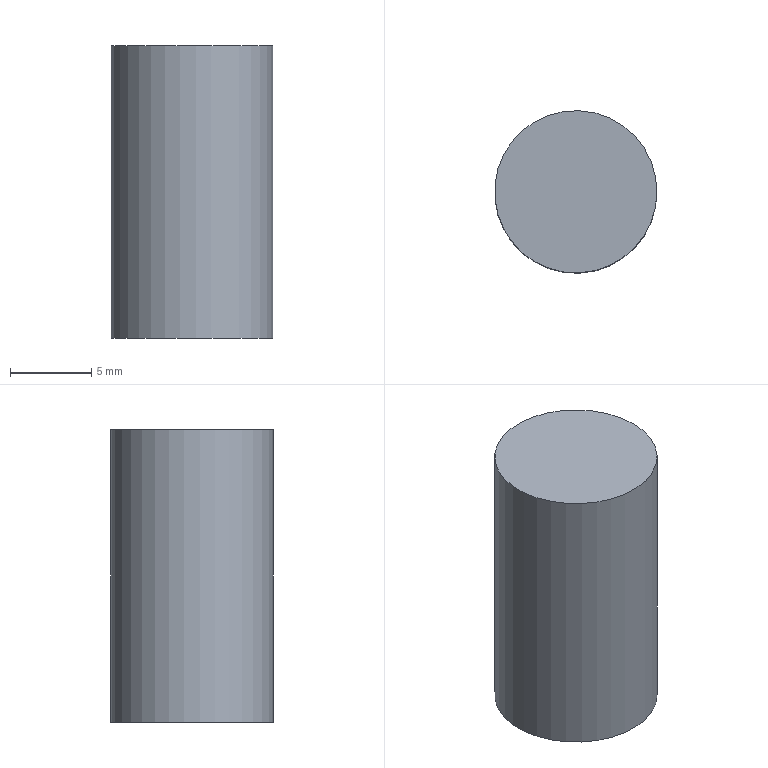Part | STEP file | xiaoding10x18 | 1 solid | 3 faces | box 10 x 10 x 18 mm | volume 1414 mm3 | plane 2 | cylinder 1 | commonest cylinder face diameters 10 x1
STEP:
#1=CARTESIAN_POINT('',(0.,0.,0.));
#2=DIRECTION('',(0.,0.,1.));
#3=DIRECTION('',(1.,0.,0.));
#4=AXIS2_PLACEMENT_3D('',#1,#2,#3);
#5=CARTESIAN_POINT('',(5.,0.,9.));
#6=VERTEX_POINT('',#5);
#7=CARTESIAN_POINT('',(0.,0.,9.));
#8=DIRECTION('',(0.,0.,1.));
#9=DIRECTION('',(1.,0.,0.));
#10=AXIS2_PLACEMENT_3D('',#7,#8,#9);
#11=CIRCLE('',#10,5.);
#12=CARTESIAN_POINT('',(0.,0.,9.));
#13=DIRECTION('',(0.,0.,-1.));
#14=DIRECTION('',(-1.,0.,0.));
#15=AXIS2_PLACEMENT_3D('',#12,#13,#14);
#16=CYLINDRICAL_SURFACE('',#15,5.);
#17=CARTESIAN_POINT('',(9.425,0.));
#18=DIRECTION('',(-1.,0.));
#19=VECTOR('',#18,1.);
#20=LINE('',#17,#19);
#21=(GEOMETRIC_REPRESENTATION_CONTEXT(2)PARAMETRIC_REPRESENTATION_CONTEXT()REPRESENTATION_CONTEXT('',''));
#22=DEFINITIONAL_REPRESENTATION('',(#20),#21);
#23=PCURVE('',#16,#22);
#24=CARTESIAN_POINT('',(0.,0.,9.));
#25=DIRECTION('',(0.,0.,1.));
#26=DIRECTION('',(1.,0.,0.));
#27=AXIS2_PLACEMENT_3D('',#24,#25,#26);
#28=PLANE('',#27);
#29=CARTESIAN_POINT('',(0.,0.));
#30=DIRECTION('',(1.,0.));
#31=AXIS2_PLACEMENT_2D('',#29,#30);
#32=CIRCLE('',#31,5.);
#33=(GEOMETRIC_REPRESENTATION_CONTEXT(2)PARAMETRIC_REPRESENTATION_CONTEXT()REPRESENTATION_CONTEXT('',''));
#34=DEFINITIONAL_REPRESENTATION('',(#32),#33);
#35=PCURVE('',#28,#34);
#36=SURFACE_CURVE('',#11,(#23,#35),.PCURVE_S1.);
#37=EDGE_CURVE('',#6,#6,#36,.T.);
#38=ORIENTED_EDGE('',*,*,#37,.F.);
#39=CARTESIAN_POINT('',(5.,0.,-9.));
#40=VERTEX_POINT('',#39);
#41=CARTESIAN_POINT('',(5.,0.,9.));
#42=CARTESIAN_POINT('',(5.,0.,-9.));
#43=B_SPLINE_CURVE_WITH_KNOTS('',1,(#41,#42),.UNSPECIFIED.,.F.,.F.,(2,2),(0.,18.),.PIECEWISE_BEZIER_KNOTS.);
#44=CARTESIAN_POINT('',(9.425,0.));
#45=DIRECTION('',(0.,1.));
#46=VECTOR('',#45,1.);
#47=LINE('',#44,#46);
#48=(GEOMETRIC_REPRESENTATION_CONTEXT(2)PARAMETRIC_REPRESENTATION_CONTEXT()REPRESENTATION_CONTEXT('',''));
#49=DEFINITIONAL_REPRESENTATION('',(#47),#48);
#50=PCURVE('',#16,#49);
#51=CARTESIAN_POINT('',(3.142,0.));
#52=DIRECTION('',(0.,1.));
#53=VECTOR('',#52,1.);
#54=LINE('',#51,#53);
#55=(GEOMETRIC_REPRESENTATION_CONTEXT(2)PARAMETRIC_REPRESENTATION_CONTEXT()REPRESENTATION_CONTEXT('',''));
#56=DEFINITIONAL_REPRESENTATION('',(#54),#55);
#57=PCURVE('',#16,#56);
#58=SEAM_CURVE('',#43,(#50,#57),.PCURVE_S1.);
#59=EDGE_CURVE('',#6,#40,#58,.T.);
#60=ORIENTED_EDGE('',*,*,#59,.T.);
#61=CARTESIAN_POINT('',(0.,0.,-9.));
#62=DIRECTION('',(0.,0.,1.));
#63=DIRECTION('',(1.,0.,0.));
#64=AXIS2_PLACEMENT_3D('',#61,#62,#63);
#65=CIRCLE('',#64,5.);
#66=CARTESIAN_POINT('',(9.425,18.));
#67=DIRECTION('',(-1.,0.));
#68=VECTOR('',#67,1.);
#69=LINE('',#66,#68);
#70=(GEOMETRIC_REPRESENTATION_CONTEXT(2)PARAMETRIC_REPRESENTATION_CONTEXT()REPRESENTATION_CONTEXT('',''));
#71=DEFINITIONAL_REPRESENTATION('',(#69),#70);
#72=PCURVE('',#16,#71);
#73=CARTESIAN_POINT('',(0.,0.,-9.));
#74=DIRECTION('',(0.,0.,1.));
#75=DIRECTION('',(1.,0.,0.));
#76=AXIS2_PLACEMENT_3D('',#73,#74,#75);
#77=PLANE('',#76);
#78=CARTESIAN_POINT('',(0.,0.));
#79=DIRECTION('',(1.,0.));
#80=AXIS2_PLACEMENT_2D('',#78,#79);
#81=CIRCLE('',#80,5.);
#82=(GEOMETRIC_REPRESENTATION_CONTEXT(2)PARAMETRIC_REPRESENTATION_CONTEXT()REPRESENTATION_CONTEXT('',''));
#83=DEFINITIONAL_REPRESENTATION('',(#81),#82);
#84=PCURVE('',#77,#83);
#85=SURFACE_CURVE('',#65,(#72,#84),.PCURVE_S1.);
#86=EDGE_CURVE('',#40,#40,#85,.T.);
#87=ORIENTED_EDGE('',*,*,#86,.T.);
#88=ORIENTED_EDGE('',*,*,#59,.F.);
#89=EDGE_LOOP('',(#38,#60,#87,#88));
#90=FACE_BOUND('',#89,.T.);
#91=ADVANCED_FACE('',(#90),#16,.T.);
#92=ORIENTED_EDGE('',*,*,#37,.T.);
#93=EDGE_LOOP('',(#92));
#94=FACE_BOUND('',#93,.T.);
#95=ADVANCED_FACE('',(#94),#28,.T.);
#96=ORIENTED_EDGE('',*,*,#86,.F.);
#97=EDGE_LOOP('',(#96));
#98=FACE_BOUND('',#97,.T.);
#99=ADVANCED_FACE('',(#98),#77,.F.);
#100=CLOSED_SHELL('',(#91,#95,#99));
#101=MANIFOLD_SOLID_BREP('',#100);
#102=(LENGTH_UNIT()NAMED_UNIT(*)SI_UNIT(.MILLI.,.METRE.));
#103=UNCERTAINTY_MEASURE_WITH_UNIT(LENGTH_MEASURE(0.00001),#102,'','');
#104=(NAMED_UNIT(*)PLANE_ANGLE_UNIT()SI_UNIT($,.RADIAN.));
#105=(NAMED_UNIT(*)SI_UNIT($,.STERADIAN.)SOLID_ANGLE_UNIT());
#106=(GEOMETRIC_REPRESENTATION_CONTEXT(3)GLOBAL_UNCERTAINTY_ASSIGNED_CONTEXT((#103))GLOBAL_UNIT_ASSIGNED_CONTEXT((#102,#104,#105))REPRESENTATION_CONTEXT('',''));
#107=ADVANCED_BREP_SHAPE_REPRESENTATION('',(#4,#101),#106);